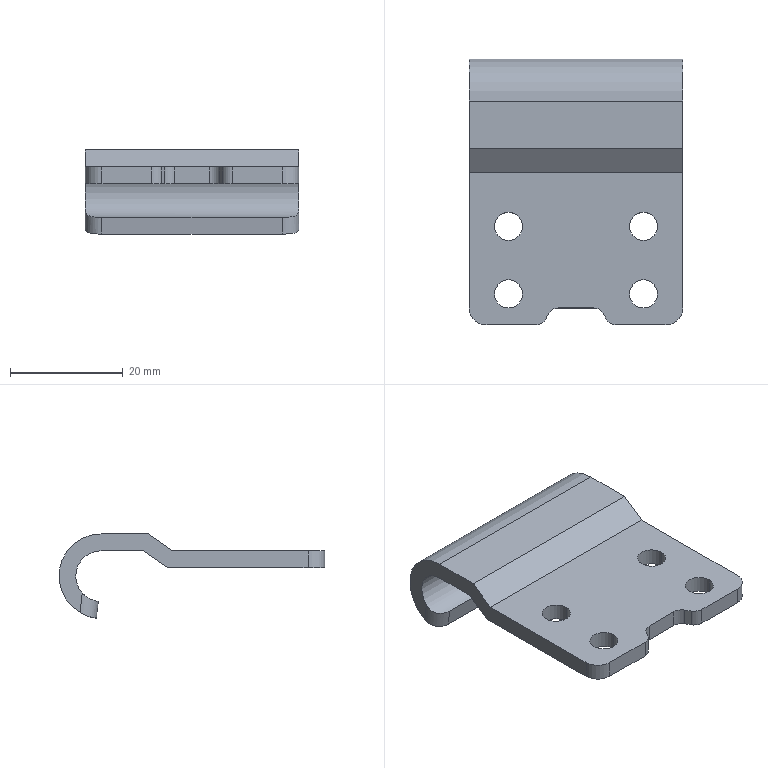Part | SolidWorks | features BaseBody 1 | 1 solid | 32 faces | box 38 x 47.284 x 14.954 mm | volume 6365 mm3 | cylinder 18 | plane 14 | commonest cylinder face diameters 5 x8 4 x4 6 x4 9 x1 15 x1
STEP:
#1=CARTESIAN_POINT('',(-19.,13.284,-5.));
#2=VERTEX_POINT('',#1);
#3=CARTESIAN_POINT('',(19.,13.284,-5.));
#4=VERTEX_POINT('',#3);
#5=CARTESIAN_POINT('',(-19.,13.284,-5.));
#6=DIRECTION('',(1.,0.,0.));
#7=VECTOR('',#6,1000.);
#8=LINE('',#5,#7);
#9=EDGE_CURVE('',#2,#4,#8,.T.);
#10=ORIENTED_EDGE('',*,*,#9,.T.);
#11=CARTESIAN_POINT('',(19.,5.784,-5.));
#12=VERTEX_POINT('',#11);
#13=CARTESIAN_POINT('',(19.,5.784,-5.));
#14=DIRECTION('',(0.,1.,0.));
#15=VECTOR('',#14,1000.);
#16=LINE('',#13,#15);
#17=EDGE_CURVE('',#12,#4,#16,.T.);
#18=ORIENTED_EDGE('',*,*,#17,.F.);
#19=CARTESIAN_POINT('',(-19.,5.784,-5.));
#20=VERTEX_POINT('',#19);
#21=CARTESIAN_POINT('',(19.,5.784,-5.));
#22=DIRECTION('',(-1.,0.,0.));
#23=VECTOR('',#22,1000.);
#24=LINE('',#21,#23);
#25=EDGE_CURVE('',#12,#20,#24,.T.);
#26=ORIENTED_EDGE('',*,*,#25,.T.);
#27=CARTESIAN_POINT('',(-19.,5.784,-5.));
#28=DIRECTION('',(0.,1.,0.));
#29=VECTOR('',#28,1000.);
#30=LINE('',#27,#29);
#31=EDGE_CURVE('',#20,#2,#30,.T.);
#32=ORIENTED_EDGE('',*,*,#31,.T.);
#33=EDGE_LOOP('',(#10,#18,#26,#32));
#34=FACE_OUTER_BOUND('',#33,.T.);
#35=CARTESIAN_POINT('',(19.,17.784,-5.));
#36=DIRECTION('',(0.,0.,-1.));
#37=DIRECTION('',(0.,-1.,0.));
#38=AXIS2_PLACEMENT_3D('',#35,#36,#37);
#39=PLANE('',#38);
#40=ADVANCED_FACE('',(#34),#39,.T.);
#41=CARTESIAN_POINT('',(-19.,-23.5,-8.));
#42=VERTEX_POINT('',#41);
#43=CARTESIAN_POINT('',(-19.,-23.5,-5.));
#44=VERTEX_POINT('',#43);
#45=CARTESIAN_POINT('',(-19.,-23.5,-8.));
#46=DIRECTION('',(0.,0.,1.));
#47=VECTOR('',#46,1000.);
#48=LINE('',#45,#47);
#49=EDGE_CURVE('',#42,#44,#48,.T.);
#50=ORIENTED_EDGE('',*,*,#49,.T.);
#51=CARTESIAN_POINT('',(-19.,0.5541,-5.));
#52=VERTEX_POINT('',#51);
#53=CARTESIAN_POINT('',(-19.,0.5541,-5.));
#54=DIRECTION('',(0.,-1.,0.));
#55=VECTOR('',#54,1000.);
#56=LINE('',#53,#55);
#57=EDGE_CURVE('',#52,#44,#56,.T.);
#58=ORIENTED_EDGE('',*,*,#57,.F.);
#59=CARTESIAN_POINT('',(-19.,4.839,-2.));
#60=VERTEX_POINT('',#59);
#61=CARTESIAN_POINT('',(-19.,4.839,-2.));
#62=DIRECTION('',(0.,-0.8192,-0.5736));
#63=VECTOR('',#62,1000.);
#64=LINE('',#61,#63);
#65=EDGE_CURVE('',#60,#52,#64,.T.);
#66=ORIENTED_EDGE('',*,*,#65,.F.);
#67=CARTESIAN_POINT('',(-19.,13.284,-2.));
#68=VERTEX_POINT('',#67);
#69=CARTESIAN_POINT('',(-19.,13.284,-2.));
#70=DIRECTION('',(0.,-1.,0.));
#71=VECTOR('',#70,1000.);
#72=LINE('',#69,#71);
#73=EDGE_CURVE('',#68,#60,#72,.T.);
#74=ORIENTED_EDGE('',*,*,#73,.F.);
#75=CARTESIAN_POINT('',(-19.,17.03,-15.998));
#76=VERTEX_POINT('',#75);
#77=CARTESIAN_POINT('',(-19.,13.284,-9.5));
#78=DIRECTION('',(1.,0.,0.));
#79=DIRECTION('',(0.,0.4994,-0.8664));
#80=AXIS2_PLACEMENT_3D('',#77,#78,#79);
#81=CIRCLE('',#80,7.5);
#82=EDGE_CURVE('',#76,#68,#81,.T.);
#83=ORIENTED_EDGE('',*,*,#82,.F.);
#84=CARTESIAN_POINT('',(-19.,16.639,-12.5));
#85=VERTEX_POINT('',#84);
#86=CARTESIAN_POINT('',(-19.,16.639,-12.5));
#87=DIRECTION('',(0.,0.1111,-0.9938));
#88=VECTOR('',#87,1000.);
#89=LINE('',#86,#88);
#90=EDGE_CURVE('',#85,#76,#89,.T.);
#91=ORIENTED_EDGE('',*,*,#90,.F.);
#92=CARTESIAN_POINT('',(-19.,13.284,-9.5));
#93=DIRECTION('',(-1.,0.,0.));
#94=DIRECTION('',(0.,0.,1.));
#95=AXIS2_PLACEMENT_3D('',#92,#93,#94);
#96=CIRCLE('',#95,4.5);
#97=EDGE_CURVE('',#2,#85,#96,.T.);
#98=ORIENTED_EDGE('',*,*,#97,.F.);
#99=ORIENTED_EDGE('',*,*,#31,.F.);
#100=CARTESIAN_POINT('',(-19.,1.5,-8.));
#101=VERTEX_POINT('',#100);
#102=CARTESIAN_POINT('',(-19.,1.5,-8.));
#103=DIRECTION('',(0.,0.8192,0.5736));
#104=VECTOR('',#103,1000.);
#105=LINE('',#102,#104);
#106=EDGE_CURVE('',#101,#20,#105,.T.);
#107=ORIENTED_EDGE('',*,*,#106,.F.);
#108=CARTESIAN_POINT('',(-19.,1.5,-8.));
#109=DIRECTION('',(0.,-1.,0.));
#110=VECTOR('',#109,1000.);
#111=LINE('',#108,#110);
#112=EDGE_CURVE('',#101,#42,#111,.T.);
#113=ORIENTED_EDGE('',*,*,#112,.T.);
#114=EDGE_LOOP('',(#50,#58,#66,#74,#83,#91,#98,#99,#107,#113));
#115=FACE_OUTER_BOUND('',#114,.T.);
#116=CARTESIAN_POINT('',(-19.,25.784,200.273));
#117=DIRECTION('',(-1.,0.,0.));
#118=DIRECTION('',(0.,0.,1.));
#119=AXIS2_PLACEMENT_3D('',#116,#117,#118);
#120=PLANE('',#119);
#121=ADVANCED_FACE('',(#115),#120,.T.);
#122=CARTESIAN_POINT('',(-9.5,-9.,-8.));
#123=VERTEX_POINT('',#122);
#124=CARTESIAN_POINT('',(-14.5,-9.,-8.));
#125=VERTEX_POINT('',#124);
#126=CARTESIAN_POINT('',(-12.,-9.,-8.));
#127=DIRECTION('',(0.,0.,-1.));
#128=DIRECTION('',(1.,0.,0.));
#129=AXIS2_PLACEMENT_3D('',#126,#127,#128);
#130=CIRCLE('',#129,2.5);
#131=EDGE_CURVE('',#123,#125,#130,.T.);
#132=ORIENTED_EDGE('',*,*,#131,.F.);
#133=CARTESIAN_POINT('',(-12.,-9.,-8.));
#134=DIRECTION('',(0.,0.,-1.));
#135=DIRECTION('',(-1.,0.,0.));
#136=AXIS2_PLACEMENT_3D('',#133,#134,#135);
#137=CIRCLE('',#136,2.5);
#138=EDGE_CURVE('',#125,#123,#137,.T.);
#139=ORIENTED_EDGE('',*,*,#138,.F.);
#140=EDGE_LOOP('',(#132,#139));
#141=FACE_BOUND('',#140,.T.);
#142=CARTESIAN_POINT('',(-9.5,-21.,-8.));
#143=VERTEX_POINT('',#142);
#144=CARTESIAN_POINT('',(-14.5,-21.,-8.));
#145=VERTEX_POINT('',#144);
#146=CARTESIAN_POINT('',(-12.,-21.,-8.));
#147=DIRECTION('',(0.,0.,-1.));
#148=DIRECTION('',(1.,0.,0.));
#149=AXIS2_PLACEMENT_3D('',#146,#147,#148);
#150=CIRCLE('',#149,2.5);
#151=EDGE_CURVE('',#143,#145,#150,.T.);
#152=ORIENTED_EDGE('',*,*,#151,.F.);
#153=CARTESIAN_POINT('',(-12.,-21.,-8.));
#154=DIRECTION('',(0.,0.,-1.));
#155=DIRECTION('',(-1.,0.,0.));
#156=AXIS2_PLACEMENT_3D('',#153,#154,#155);
#157=CIRCLE('',#156,2.5);
#158=EDGE_CURVE('',#145,#143,#157,.T.);
#159=ORIENTED_EDGE('',*,*,#158,.F.);
#160=EDGE_LOOP('',(#152,#159));
#161=FACE_BOUND('',#160,.T.);
#162=CARTESIAN_POINT('',(14.5,-9.,-8.));
#163=VERTEX_POINT('',#162);
#164=CARTESIAN_POINT('',(9.5,-9.,-8.));
#165=VERTEX_POINT('',#164);
#166=CARTESIAN_POINT('',(12.,-9.,-8.));
#167=DIRECTION('',(0.,0.,-1.));
#168=DIRECTION('',(1.,0.,0.));
#169=AXIS2_PLACEMENT_3D('',#166,#167,#168);
#170=CIRCLE('',#169,2.5);
#171=EDGE_CURVE('',#163,#165,#170,.T.);
#172=ORIENTED_EDGE('',*,*,#171,.F.);
#173=CARTESIAN_POINT('',(12.,-9.,-8.));
#174=DIRECTION('',(0.,0.,-1.));
#175=DIRECTION('',(-1.,0.,0.));
#176=AXIS2_PLACEMENT_3D('',#173,#174,#175);
#177=CIRCLE('',#176,2.5);
#178=EDGE_CURVE('',#165,#163,#177,.T.);
#179=ORIENTED_EDGE('',*,*,#178,.F.);
#180=EDGE_LOOP('',(#172,#179));
#181=FACE_BOUND('',#180,.T.);
#182=CARTESIAN_POINT('',(14.5,-21.,-8.));
#183=VERTEX_POINT('',#182);
#184=CARTESIAN_POINT('',(9.5,-21.,-8.));
#185=VERTEX_POINT('',#184);
#186=CARTESIAN_POINT('',(12.,-21.,-8.));
#187=DIRECTION('',(0.,0.,-1.));
#188=DIRECTION('',(1.,0.,0.));
#189=AXIS2_PLACEMENT_3D('',#186,#187,#188);
#190=CIRCLE('',#189,2.5);
#191=EDGE_CURVE('',#183,#185,#190,.T.);
#192=ORIENTED_EDGE('',*,*,#191,.F.);
#193=CARTESIAN_POINT('',(12.,-21.,-8.));
#194=DIRECTION('',(0.,0.,-1.));
#195=DIRECTION('',(-1.,0.,0.));
#196=AXIS2_PLACEMENT_3D('',#193,#194,#195);
#197=CIRCLE('',#196,2.5);
#198=EDGE_CURVE('',#185,#183,#197,.T.);
#199=ORIENTED_EDGE('',*,*,#198,.F.);
#200=EDGE_LOOP('',(#192,#199));
#201=FACE_BOUND('',#200,.T.);
#202=CARTESIAN_POINT('',(-16.,-26.5,-8.));
#203=VERTEX_POINT('',#202);
#204=CARTESIAN_POINT('',(-16.,-23.5,-8.));
#205=DIRECTION('',(0.,0.,1.));
#206=DIRECTION('',(-1.,0.,0.));
#207=AXIS2_PLACEMENT_3D('',#204,#205,#206);
#208=CIRCLE('',#207,3.);
#209=EDGE_CURVE('',#42,#203,#208,.T.);
#210=ORIENTED_EDGE('',*,*,#209,.F.);
#211=ORIENTED_EDGE('',*,*,#112,.F.);
#212=CARTESIAN_POINT('',(19.,1.5,-8.));
#213=VERTEX_POINT('',#212);
#214=CARTESIAN_POINT('',(19.,1.5,-8.));
#215=DIRECTION('',(-1.,0.,0.));
#216=VECTOR('',#215,1000.);
#217=LINE('',#214,#216);
#218=EDGE_CURVE('',#213,#101,#217,.T.);
#219=ORIENTED_EDGE('',*,*,#218,.F.);
#220=CARTESIAN_POINT('',(19.,-23.5,-8.));
#221=VERTEX_POINT('',#220);
#222=CARTESIAN_POINT('',(19.,-23.5,-8.));
#223=DIRECTION('',(0.,1.,0.));
#224=VECTOR('',#223,1000.);
#225=LINE('',#222,#224);
#226=EDGE_CURVE('',#221,#213,#225,.T.);
#227=ORIENTED_EDGE('',*,*,#226,.F.);
#228=CARTESIAN_POINT('',(16.,-26.5,-8.));
#229=VERTEX_POINT('',#228);
#230=CARTESIAN_POINT('',(16.,-23.5,-8.));
#231=DIRECTION('',(0.,0.,1.));
#232=DIRECTION('',(0.,-1.,0.));
#233=AXIS2_PLACEMENT_3D('',#230,#231,#232);
#234=CIRCLE('',#233,3.);
#235=EDGE_CURVE('',#229,#221,#234,.T.);
#236=ORIENTED_EDGE('',*,*,#235,.F.);
#237=CARTESIAN_POINT('',(7.155,-26.5,-8.));
#238=VERTEX_POINT('',#237);
#239=CARTESIAN_POINT('',(7.155,-26.5,-8.));
#240=DIRECTION('',(1.,0.,0.));
#241=VECTOR('',#240,1000.);
#242=LINE('',#239,#241);
#243=EDGE_CURVE('',#238,#229,#242,.T.);
#244=ORIENTED_EDGE('',*,*,#243,.F.);
#245=CARTESIAN_POINT('',(5.423,-25.5,-8.));
#246=VERTEX_POINT('',#245);
#247=CARTESIAN_POINT('',(7.155,-24.5,-8.));
#248=DIRECTION('',(0.,0.,1.));
#249=DIRECTION('',(-0.866,-0.5,0.));
#250=AXIS2_PLACEMENT_3D('',#247,#248,#249);
#251=CIRCLE('',#250,2.);
#252=EDGE_CURVE('',#246,#238,#251,.T.);
#253=ORIENTED_EDGE('',*,*,#252,.F.);
#254=CARTESIAN_POINT('',(4.845,-24.5,-8.));
#255=VERTEX_POINT('',#254);
#256=CARTESIAN_POINT('',(4.845,-24.5,-8.));
#257=DIRECTION('',(0.5,-0.866,0.));
#258=VECTOR('',#257,1000.);
#259=LINE('',#256,#258);
#260=EDGE_CURVE('',#255,#246,#259,.T.);
#261=ORIENTED_EDGE('',*,*,#260,.F.);
#262=CARTESIAN_POINT('',(3.113,-23.5,-8.));
#263=VERTEX_POINT('',#262);
#264=CARTESIAN_POINT('',(3.113,-25.5,-8.));
#265=DIRECTION('',(0.,0.,-1.));
#266=DIRECTION('',(0.,1.,0.));
#267=AXIS2_PLACEMENT_3D('',#264,#265,#266);
#268=CIRCLE('',#267,2.);
#269=EDGE_CURVE('',#263,#255,#268,.T.);
#270=ORIENTED_EDGE('',*,*,#269,.F.);
#271=CARTESIAN_POINT('',(-3.113,-23.5,-8.));
#272=VERTEX_POINT('',#271);
#273=CARTESIAN_POINT('',(-3.113,-23.5,-8.));
#274=DIRECTION('',(1.,0.,0.));
#275=VECTOR('',#274,1000.);
#276=LINE('',#273,#275);
#277=EDGE_CURVE('',#272,#263,#276,.T.);
#278=ORIENTED_EDGE('',*,*,#277,.F.);
#279=CARTESIAN_POINT('',(-4.845,-24.5,-8.));
#280=VERTEX_POINT('',#279);
#281=CARTESIAN_POINT('',(-3.113,-25.5,-8.));
#282=DIRECTION('',(0.,0.,-1.));
#283=DIRECTION('',(-0.866,0.5,0.));
#284=AXIS2_PLACEMENT_3D('',#281,#282,#283);
#285=CIRCLE('',#284,2.);
#286=EDGE_CURVE('',#280,#272,#285,.T.);
#287=ORIENTED_EDGE('',*,*,#286,.F.);
#288=CARTESIAN_POINT('',(-5.423,-25.5,-8.));
#289=VERTEX_POINT('',#288);
#290=CARTESIAN_POINT('',(-5.423,-25.5,-8.));
#291=DIRECTION('',(0.5,0.866,0.));
#292=VECTOR('',#291,1000.);
#293=LINE('',#290,#292);
#294=EDGE_CURVE('',#289,#280,#293,.T.);
#295=ORIENTED_EDGE('',*,*,#294,.F.);
#296=CARTESIAN_POINT('',(-7.155,-26.5,-8.));
#297=VERTEX_POINT('',#296);
#298=CARTESIAN_POINT('',(-7.155,-24.5,-8.));
#299=DIRECTION('',(0.,0.,1.));
#300=DIRECTION('',(0.,-1.,0.));
#301=AXIS2_PLACEMENT_3D('',#298,#299,#300);
#302=CIRCLE('',#301,2.);
#303=EDGE_CURVE('',#297,#289,#302,.T.);
#304=ORIENTED_EDGE('',*,*,#303,.F.);
#305=CARTESIAN_POINT('',(-16.,-26.5,-8.));
#306=DIRECTION('',(1.,0.,0.));
#307=VECTOR('',#306,1000.);
#308=LINE('',#305,#307);
#309=EDGE_CURVE('',#203,#297,#308,.T.);
#310=ORIENTED_EDGE('',*,*,#309,.F.);
#311=EDGE_LOOP('',(#210,#211,#219,#227,#236,#244,#253,#261,#270,#278,#287,#295,#304,#310));
#312=FACE_OUTER_BOUND('',#311,.T.);
#313=CARTESIAN_POINT('',(19.,1.5,-8.));
#314=DIRECTION('',(0.,0.,-1.));
#315=DIRECTION('',(0.,-1.,0.));
#316=AXIS2_PLACEMENT_3D('',#313,#314,#315);
#317=PLANE('',#316);
#318=ADVANCED_FACE('',(#141,#161,#181,#201,#312),#317,.T.);
#319=CARTESIAN_POINT('',(-16.,-26.5,-5.));
#320=VERTEX_POINT('',#319);
#321=CARTESIAN_POINT('',(-16.,-26.5,-5.));
#322=DIRECTION('',(0.,0.,-1.));
#323=VECTOR('',#322,1000.);
#324=LINE('',#321,#323);
#325=EDGE_CURVE('',#320,#203,#324,.T.);
#326=ORIENTED_EDGE('',*,*,#325,.T.);
#327=ORIENTED_EDGE('',*,*,#309,.T.);
#328=CARTESIAN_POINT('',(-7.155,-26.5,-5.));
#329=VERTEX_POINT('',#328);
#330=CARTESIAN_POINT('',(-7.155,-26.5,-8.));
#331=DIRECTION('',(0.,0.,1.));
#332=VECTOR('',#331,1000.);
#333=LINE('',#330,#332);
#334=EDGE_CURVE('',#297,#329,#333,.T.);
#335=ORIENTED_EDGE('',*,*,#334,.T.);
#336=CARTESIAN_POINT('',(-16.,-26.5,-5.));
#337=DIRECTION('',(1.,0.,0.));
#338=VECTOR('',#337,1000.);
#339=LINE('',#336,#338);
#340=EDGE_CURVE('',#320,#329,#339,.T.);
#341=ORIENTED_EDGE('',*,*,#340,.F.);
#342=EDGE_LOOP('',(#326,#327,#335,#341));
#343=FACE_OUTER_BOUND('',#342,.T.);
#344=CARTESIAN_POINT('',(19.,-26.5,-8.));
#345=DIRECTION('',(0.,-1.,0.));
#346=DIRECTION('',(0.,0.,-1.));
#347=AXIS2_PLACEMENT_3D('',#344,#345,#346);
#348=PLANE('',#347);
#349=ADVANCED_FACE('',(#343),#348,.T.);
#350=CARTESIAN_POINT('',(-9.5,-9.,-5.));
#351=VERTEX_POINT('',#350);
#352=CARTESIAN_POINT('',(-14.5,-9.,-5.));
#353=VERTEX_POINT('',#352);
#354=CARTESIAN_POINT('',(-12.,-9.,-5.));
#355=DIRECTION('',(0.,0.,1.));
#356=DIRECTION('',(1.,0.,0.));
#357=AXIS2_PLACEMENT_3D('',#354,#355,#356);
#358=CIRCLE('',#357,2.5);
#359=EDGE_CURVE('',#351,#353,#358,.T.);
#360=ORIENTED_EDGE('',*,*,#359,.F.);
#361=CARTESIAN_POINT('',(-12.,-9.,-5.));
#362=DIRECTION('',(0.,0.,1.));
#363=DIRECTION('',(-1.,0.,0.));
#364=AXIS2_PLACEMENT_3D('',#361,#362,#363);
#365=CIRCLE('',#364,2.5);
#366=EDGE_CURVE('',#353,#351,#365,.T.);
#367=ORIENTED_EDGE('',*,*,#366,.F.);
#368=EDGE_LOOP('',(#360,#367));
#369=FACE_BOUND('',#368,.T.);
#370=CARTESIAN_POINT('',(-9.5,-21.,-5.));
#371=VERTEX_POINT('',#370);
#372=CARTESIAN_POINT('',(-14.5,-21.,-5.));
#373=VERTEX_POINT('',#372);
#374=CARTESIAN_POINT('',(-12.,-21.,-5.));
#375=DIRECTION('',(0.,0.,1.));
#376=DIRECTION('',(1.,0.,0.));
#377=AXIS2_PLACEMENT_3D('',#374,#375,#376);
#378=CIRCLE('',#377,2.5);
#379=EDGE_CURVE('',#371,#373,#378,.T.);
#380=ORIENTED_EDGE('',*,*,#379,.F.);
#381=CARTESIAN_POINT('',(-12.,-21.,-5.));
#382=DIRECTION('',(0.,0.,1.));
#383=DIRECTION('',(-1.,0.,0.));
#384=AXIS2_PLACEMENT_3D('',#381,#382,#383);
#385=CIRCLE('',#384,2.5);
#386=EDGE_CURVE('',#373,#371,#385,.T.);
#387=ORIENTED_EDGE('',*,*,#386,.F.);
#388=EDGE_LOOP('',(#380,#387));
#389=FACE_BOUND('',#388,.T.);
#390=CARTESIAN_POINT('',(14.5,-9.,-5.));
#391=VERTEX_POINT('',#390);
#392=CARTESIAN_POINT('',(9.5,-9.,-5.));
#393=VERTEX_POINT('',#392);
#394=CARTESIAN_POINT('',(12.,-9.,-5.));
#395=DIRECTION('',(0.,0.,1.));
#396=DIRECTION('',(1.,0.,0.));
#397=AXIS2_PLACEMENT_3D('',#394,#395,#396);
#398=CIRCLE('',#397,2.5);
#399=EDGE_CURVE('',#391,#393,#398,.T.);
#400=ORIENTED_EDGE('',*,*,#399,.F.);
#401=CARTESIAN_POINT('',(12.,-9.,-5.));
#402=DIRECTION('',(0.,0.,1.));
#403=DIRECTION('',(-1.,0.,0.));
#404=AXIS2_PLACEMENT_3D('',#401,#402,#403);
#405=CIRCLE('',#404,2.5);
#406=EDGE_CURVE('',#393,#391,#405,.T.);
#407=ORIENTED_EDGE('',*,*,#406,.F.);
#408=EDGE_LOOP('',(#400,#407));
#409=FACE_BOUND('',#408,.T.);
#410=CARTESIAN_POINT('',(14.5,-21.,-5.));
#411=VERTEX_POINT('',#410);
#412=CARTESIAN_POINT('',(9.5,-21.,-5.));
#413=VERTEX_POINT('',#412);
#414=CARTESIAN_POINT('',(12.,-21.,-5.));
#415=DIRECTION('',(0.,0.,1.));
#416=DIRECTION('',(1.,0.,0.));
#417=AXIS2_PLACEMENT_3D('',#414,#415,#416);
#418=CIRCLE('',#417,2.5);
#419=EDGE_CURVE('',#411,#413,#418,.T.);
#420=ORIENTED_EDGE('',*,*,#419,.F.);
#421=CARTESIAN_POINT('',(12.,-21.,-5.));
#422=DIRECTION('',(0.,0.,1.));
#423=DIRECTION('',(-1.,0.,0.));
#424=AXIS2_PLACEMENT_3D('',#421,#422,#423);
#425=CIRCLE('',#424,2.5);
#426=EDGE_CURVE('',#413,#411,#425,.T.);
#427=ORIENTED_EDGE('',*,*,#426,.F.);
#428=EDGE_LOOP('',(#420,#427));
#429=FACE_BOUND('',#428,.T.);
#430=CARTESIAN_POINT('',(-16.,-23.5,-5.));
#431=DIRECTION('',(0.,0.,-1.));
#432=DIRECTION('',(0.,-1.,0.));
#433=AXIS2_PLACEMENT_3D('',#430,#431,#432);
#434=CIRCLE('',#433,3.);
#435=EDGE_CURVE('',#320,#44,#434,.T.);
#436=ORIENTED_EDGE('',*,*,#435,.F.);
#437=ORIENTED_EDGE('',*,*,#340,.T.);
#438=CARTESIAN_POINT('',(-5.423,-25.5,-5.));
#439=VERTEX_POINT('',#438);
#440=CARTESIAN_POINT('',(-7.155,-24.5,-5.));
#441=DIRECTION('',(0.,0.,-1.));
#442=DIRECTION('',(0.866,-0.5,0.));
#443=AXIS2_PLACEMENT_3D('',#440,#441,#442);
#444=CIRCLE('',#443,2.);
#445=EDGE_CURVE('',#439,#329,#444,.T.);
#446=ORIENTED_EDGE('',*,*,#445,.F.);
#447=CARTESIAN_POINT('',(-4.845,-24.5,-5.));
#448=VERTEX_POINT('',#447);
#449=CARTESIAN_POINT('',(-4.845,-24.5,-5.));
#450=DIRECTION('',(-0.5,-0.866,0.));
#451=VECTOR('',#450,1000.);
#452=LINE('',#449,#451);
#453=EDGE_CURVE('',#448,#439,#452,.T.);
#454=ORIENTED_EDGE('',*,*,#453,.F.);
#455=CARTESIAN_POINT('',(-3.113,-23.5,-5.));
#456=VERTEX_POINT('',#455);
#457=CARTESIAN_POINT('',(-3.113,-25.5,-5.));
#458=DIRECTION('',(0.,0.,1.));
#459=DIRECTION('',(0.,1.,0.));
#460=AXIS2_PLACEMENT_3D('',#457,#458,#459);
#461=CIRCLE('',#460,2.);
#462=EDGE_CURVE('',#456,#448,#461,.T.);
#463=ORIENTED_EDGE('',*,*,#462,.F.);
#464=CARTESIAN_POINT('',(3.113,-23.5,-5.));
#465=VERTEX_POINT('',#464);
#466=CARTESIAN_POINT('',(3.113,-23.5,-5.));
#467=DIRECTION('',(-1.,0.,0.));
#468=VECTOR('',#467,1000.);
#469=LINE('',#466,#468);
#470=EDGE_CURVE('',#465,#456,#469,.T.);
#471=ORIENTED_EDGE('',*,*,#470,.F.);
#472=CARTESIAN_POINT('',(4.845,-24.5,-5.));
#473=VERTEX_POINT('',#472);
#474=CARTESIAN_POINT('',(3.113,-25.5,-5.));
#475=DIRECTION('',(0.,0.,1.));
#476=DIRECTION('',(0.866,0.5,0.));
#477=AXIS2_PLACEMENT_3D('',#474,#475,#476);
#478=CIRCLE('',#477,2.);
#479=EDGE_CURVE('',#473,#465,#478,.T.);
#480=ORIENTED_EDGE('',*,*,#479,.F.);
#481=CARTESIAN_POINT('',(5.423,-25.5,-5.));
#482=VERTEX_POINT('',#481);
#483=CARTESIAN_POINT('',(5.423,-25.5,-5.));
#484=DIRECTION('',(-0.5,0.866,0.));
#485=VECTOR('',#484,1000.);
#486=LINE('',#483,#485);
#487=EDGE_CURVE('',#482,#473,#486,.T.);
#488=ORIENTED_EDGE('',*,*,#487,.F.);
#489=CARTESIAN_POINT('',(7.155,-26.5,-5.));
#490=VERTEX_POINT('',#489);
#491=CARTESIAN_POINT('',(7.155,-24.5,-5.));
#492=DIRECTION('',(0.,0.,-1.));
#493=DIRECTION('',(0.,-1.,0.));
#494=AXIS2_PLACEMENT_3D('',#491,#492,#493);
#495=CIRCLE('',#494,2.);
#496=EDGE_CURVE('',#490,#482,#495,.T.);
#497=ORIENTED_EDGE('',*,*,#496,.F.);
#498=CARTESIAN_POINT('',(16.,-26.5,-5.));
#499=VERTEX_POINT('',#498);
#500=CARTESIAN_POINT('',(7.155,-26.5,-5.));
#501=DIRECTION('',(1.,0.,0.));
#502=VECTOR('',#501,1000.);
#503=LINE('',#500,#502);
#504=EDGE_CURVE('',#490,#499,#503,.T.);
#505=ORIENTED_EDGE('',*,*,#504,.T.);
#506=CARTESIAN_POINT('',(19.,-23.5,-5.));
#507=VERTEX_POINT('',#506);
#508=CARTESIAN_POINT('',(16.,-23.5,-5.));
#509=DIRECTION('',(0.,0.,-1.));
#510=DIRECTION('',(1.,0.,0.));
#511=AXIS2_PLACEMENT_3D('',#508,#509,#510);
#512=CIRCLE('',#511,3.);
#513=EDGE_CURVE('',#507,#499,#512,.T.);
#514=ORIENTED_EDGE('',*,*,#513,.F.);
#515=CARTESIAN_POINT('',(19.,0.5541,-5.));
#516=VERTEX_POINT('',#515);
#517=CARTESIAN_POINT('',(19.,0.5541,-5.));
#518=DIRECTION('',(0.,-1.,0.));
#519=VECTOR('',#518,1000.);
#520=LINE('',#517,#519);
#521=EDGE_CURVE('',#516,#507,#520,.T.);
#522=ORIENTED_EDGE('',*,*,#521,.F.);
#523=CARTESIAN_POINT('',(-19.,0.5541,-5.));
#524=DIRECTION('',(1.,0.,0.));
#525=VECTOR('',#524,1000.);
#526=LINE('',#523,#525);
#527=EDGE_CURVE('',#52,#516,#526,.T.);
#528=ORIENTED_EDGE('',*,*,#527,.F.);
#529=ORIENTED_EDGE('',*,*,#57,.T.);
#530=EDGE_LOOP('',(#436,#437,#446,#454,#463,#471,#480,#488,#497,#505,#514,#522,#528,#529));
#531=FACE_OUTER_BOUND('',#530,.T.);
#532=CARTESIAN_POINT('',(19.,-26.5,-5.));
#533=DIRECTION('',(0.,0.,1.));
#534=DIRECTION('',(1.,0.,0.));
#535=AXIS2_PLACEMENT_3D('',#532,#533,#534);
#536=PLANE('',#535);
#537=ADVANCED_FACE('',(#369,#389,#409,#429,#531),#536,.T.);
#538=CARTESIAN_POINT('',(19.,4.839,-2.));
#539=VERTEX_POINT('',#538);
#540=CARTESIAN_POINT('',(19.,0.5541,-5.));
#541=DIRECTION('',(0.,0.8192,0.5736));
#542=VECTOR('',#541,1000.);
#543=LINE('',#540,#542);
#544=EDGE_CURVE('',#516,#539,#543,.T.);
#545=ORIENTED_EDGE('',*,*,#544,.T.);
#546=CARTESIAN_POINT('',(19.,4.839,-2.));
#547=DIRECTION('',(-1.,0.,0.));
#548=VECTOR('',#547,1000.);
#549=LINE('',#546,#548);
#550=EDGE_CURVE('',#539,#60,#549,.T.);
#551=ORIENTED_EDGE('',*,*,#550,.T.);
#552=ORIENTED_EDGE('',*,*,#65,.T.);
#553=ORIENTED_EDGE('',*,*,#527,.T.);
#554=EDGE_LOOP('',(#545,#551,#552,#553));
#555=FACE_OUTER_BOUND('',#554,.T.);
#556=CARTESIAN_POINT('',(19.,0.5541,-5.));
#557=DIRECTION('',(0.,-0.5736,0.8192));
#558=DIRECTION('',(-1.,0.,0.));
#559=AXIS2_PLACEMENT_3D('',#556,#557,#558);
#560=PLANE('',#559);
#561=ADVANCED_FACE('',(#555),#560,.T.);
#562=CARTESIAN_POINT('',(19.,13.284,-2.));
#563=VERTEX_POINT('',#562);
#564=CARTESIAN_POINT('',(19.,13.284,-2.));
#565=DIRECTION('',(-1.,0.,0.));
#566=VECTOR('',#565,1000.);
#567=LINE('',#564,#566);
#568=EDGE_CURVE('',#563,#68,#567,.T.);
#569=ORIENTED_EDGE('',*,*,#568,.T.);
#570=ORIENTED_EDGE('',*,*,#73,.T.);
#571=ORIENTED_EDGE('',*,*,#550,.F.);
#572=CARTESIAN_POINT('',(19.,13.284,-2.));
#573=DIRECTION('',(0.,-1.,0.));
#574=VECTOR('',#573,1000.);
#575=LINE('',#572,#574);
#576=EDGE_CURVE('',#563,#539,#575,.T.);
#577=ORIENTED_EDGE('',*,*,#576,.F.);
#578=EDGE_LOOP('',(#569,#570,#571,#577));
#579=FACE_OUTER_BOUND('',#578,.T.);
#580=CARTESIAN_POINT('',(19.,4.839,-2.));
#581=DIRECTION('',(0.,0.,1.));
#582=DIRECTION('',(1.,0.,0.));
#583=AXIS2_PLACEMENT_3D('',#580,#581,#582);
#584=PLANE('',#583);
#585=ADVANCED_FACE('',(#579),#584,.T.);
#586=ORIENTED_EDGE('',*,*,#17,.T.);
#587=CARTESIAN_POINT('',(19.,16.639,-12.5));
#588=VERTEX_POINT('',#587);
#589=CARTESIAN_POINT('',(19.,13.284,-9.5));
#590=DIRECTION('',(1.,0.,0.));
#591=DIRECTION('',(0.,0.7454,-0.6667));
#592=AXIS2_PLACEMENT_3D('',#589,#590,#591);
#593=CIRCLE('',#592,4.5);
#594=EDGE_CURVE('',#588,#4,#593,.T.);
#595=ORIENTED_EDGE('',*,*,#594,.F.);
#596=CARTESIAN_POINT('',(19.,17.03,-15.998));
#597=VERTEX_POINT('',#596);
#598=CARTESIAN_POINT('',(19.,17.03,-15.998));
#599=DIRECTION('',(0.,-0.1111,0.9938));
#600=VECTOR('',#599,1000.);
#601=LINE('',#598,#600);
#602=EDGE_CURVE('',#597,#588,#601,.T.);
#603=ORIENTED_EDGE('',*,*,#602,.F.);
#604=CARTESIAN_POINT('',(19.,13.284,-9.5));
#605=DIRECTION('',(-1.,0.,0.));
#606=DIRECTION('',(0.,0.,1.));
#607=AXIS2_PLACEMENT_3D('',#604,#605,#606);
#608=CIRCLE('',#607,7.5);
#609=EDGE_CURVE('',#563,#597,#608,.T.);
#610=ORIENTED_EDGE('',*,*,#609,.F.);
#611=ORIENTED_EDGE('',*,*,#576,.T.);
#612=ORIENTED_EDGE('',*,*,#544,.F.);
#613=ORIENTED_EDGE('',*,*,#521,.T.);
#614=CARTESIAN_POINT('',(19.,-23.5,-5.));
#615=DIRECTION('',(0.,0.,-1.));
#616=VECTOR('',#615,1000.);
#617=LINE('',#614,#616);
#618=EDGE_CURVE('',#507,#221,#617,.T.);
#619=ORIENTED_EDGE('',*,*,#618,.T.);
#620=ORIENTED_EDGE('',*,*,#226,.T.);
#621=CARTESIAN_POINT('',(19.,5.784,-5.));
#622=DIRECTION('',(0.,-0.8192,-0.5736));
#623=VECTOR('',#622,1000.);
#624=LINE('',#621,#623);
#625=EDGE_CURVE('',#12,#213,#624,.T.);
#626=ORIENTED_EDGE('',*,*,#625,.F.);
#627=EDGE_LOOP('',(#586,#595,#603,#610,#611,#612,#613,#619,#620,#626));
#628=FACE_OUTER_BOUND('',#627,.T.);
#629=CARTESIAN_POINT('',(19.,25.784,200.273));
#630=DIRECTION('',(-1.,0.,0.));
#631=DIRECTION('',(0.,0.,1.));
#632=AXIS2_PLACEMENT_3D('',#629,#630,#631);
#633=PLANE('',#632);
#634=ADVANCED_FACE('',(#628),#633,.F.);
#635=ORIENTED_EDGE('',*,*,#625,.T.);
#636=ORIENTED_EDGE('',*,*,#218,.T.);
#637=ORIENTED_EDGE('',*,*,#106,.T.);
#638=ORIENTED_EDGE('',*,*,#25,.F.);
#639=EDGE_LOOP('',(#635,#636,#637,#638));
#640=FACE_OUTER_BOUND('',#639,.T.);
#641=CARTESIAN_POINT('',(19.,5.784,-5.));
#642=DIRECTION('',(0.,0.5736,-0.8192));
#643=DIRECTION('',(-1.,0.,0.));
#644=AXIS2_PLACEMENT_3D('',#641,#642,#643);
#645=PLANE('',#644);
#646=ADVANCED_FACE('',(#640),#645,.T.);
#647=CARTESIAN_POINT('',(16.,-26.5,-8.));
#648=DIRECTION('',(0.,0.,1.));
#649=VECTOR('',#648,1000.);
#650=LINE('',#647,#649);
#651=EDGE_CURVE('',#229,#499,#650,.T.);
#652=ORIENTED_EDGE('',*,*,#651,.F.);
#653=ORIENTED_EDGE('',*,*,#235,.T.);
#654=ORIENTED_EDGE('',*,*,#618,.F.);
#655=ORIENTED_EDGE('',*,*,#513,.T.);
#656=EDGE_LOOP('',(#652,#653,#654,#655));
#657=FACE_OUTER_BOUND('',#656,.T.);
#658=CARTESIAN_POINT('',(16.,-23.5,-4.463));
#659=DIRECTION('',(0.,0.,-1.));
#660=DIRECTION('',(1.,0.,0.));
#661=AXIS2_PLACEMENT_3D('',#658,#659,#660);
#662=CYLINDRICAL_SURFACE('',#661,3.);
#663=ADVANCED_FACE('',(#657),#662,.T.);
#664=ORIENTED_EDGE('',*,*,#651,.T.);
#665=ORIENTED_EDGE('',*,*,#504,.F.);
#666=CARTESIAN_POINT('',(7.155,-26.5,-5.));
#667=DIRECTION('',(0.,0.,-1.));
#668=VECTOR('',#667,1000.);
#669=LINE('',#666,#668);
#670=EDGE_CURVE('',#490,#238,#669,.T.);
#671=ORIENTED_EDGE('',*,*,#670,.T.);
#672=ORIENTED_EDGE('',*,*,#243,.T.);
#673=EDGE_LOOP('',(#664,#665,#671,#672));
#674=FACE_OUTER_BOUND('',#673,.T.);
#675=CARTESIAN_POINT('',(19.,-26.5,-8.));
#676=DIRECTION('',(0.,-1.,0.));
#677=DIRECTION('',(0.,0.,-1.));
#678=AXIS2_PLACEMENT_3D('',#675,#676,#677);
#679=PLANE('',#678);
#680=ADVANCED_FACE('',(#674),#679,.T.);
#681=CARTESIAN_POINT('',(5.423,-25.5,-8.));
#682=DIRECTION('',(0.,0.,1.));
#683=VECTOR('',#682,1000.);
#684=LINE('',#681,#683);
#685=EDGE_CURVE('',#246,#482,#684,.T.);
#686=ORIENTED_EDGE('',*,*,#685,.F.);
#687=ORIENTED_EDGE('',*,*,#252,.T.);
#688=ORIENTED_EDGE('',*,*,#670,.F.);
#689=ORIENTED_EDGE('',*,*,#496,.T.);
#690=EDGE_LOOP('',(#686,#687,#688,#689));
#691=FACE_OUTER_BOUND('',#690,.T.);
#692=CARTESIAN_POINT('',(7.155,-24.5,-4.672));
#693=DIRECTION('',(0.,0.,-1.));
#694=DIRECTION('',(1.,0.,0.));
#695=AXIS2_PLACEMENT_3D('',#692,#693,#694);
#696=CYLINDRICAL_SURFACE('',#695,2.);
#697=ADVANCED_FACE('',(#691),#696,.T.);
#698=ORIENTED_EDGE('',*,*,#260,.T.);
#699=ORIENTED_EDGE('',*,*,#685,.T.);
#700=ORIENTED_EDGE('',*,*,#487,.T.);
#701=CARTESIAN_POINT('',(4.845,-24.5,-5.));
#702=DIRECTION('',(0.,0.,-1.));
#703=VECTOR('',#702,1000.);
#704=LINE('',#701,#703);
#705=EDGE_CURVE('',#473,#255,#704,.T.);
#706=ORIENTED_EDGE('',*,*,#705,.T.);
#707=EDGE_LOOP('',(#698,#699,#700,#706));
#708=FACE_OUTER_BOUND('',#707,.T.);
#709=CARTESIAN_POINT('',(4.268,-23.5,-8.));
#710=DIRECTION('',(0.866,0.5,0.));
#711=DIRECTION('',(0.,0.,-1.));
#712=AXIS2_PLACEMENT_3D('',#709,#710,#711);
#713=PLANE('',#712);
#714=ADVANCED_FACE('',(#708),#713,.F.);
#715=ORIENTED_EDGE('',*,*,#269,.T.);
#716=ORIENTED_EDGE('',*,*,#705,.F.);
#717=ORIENTED_EDGE('',*,*,#479,.T.);
#718=CARTESIAN_POINT('',(3.113,-23.5,-8.));
#719=DIRECTION('',(0.,0.,1.));
#720=VECTOR('',#719,1000.);
#721=LINE('',#718,#720);
#722=EDGE_CURVE('',#263,#465,#721,.T.);
#723=ORIENTED_EDGE('',*,*,#722,.F.);
#724=EDGE_LOOP('',(#715,#716,#717,#723));
#725=FACE_OUTER_BOUND('',#724,.T.);
#726=CARTESIAN_POINT('',(3.113,-25.5,-8.384));
#727=DIRECTION('',(0.,0.,1.));
#728=DIRECTION('',(-1.,0.,0.));
#729=AXIS2_PLACEMENT_3D('',#726,#727,#728);
#730=CYLINDRICAL_SURFACE('',#729,2.);
#731=ADVANCED_FACE('',(#725),#730,.F.);
#732=ORIENTED_EDGE('',*,*,#277,.T.);
#733=ORIENTED_EDGE('',*,*,#722,.T.);
#734=ORIENTED_EDGE('',*,*,#470,.T.);
#735=CARTESIAN_POINT('',(-3.113,-23.5,-5.));
#736=DIRECTION('',(0.,0.,-1.));
#737=VECTOR('',#736,1000.);
#738=LINE('',#735,#737);
#739=EDGE_CURVE('',#456,#272,#738,.T.);
#740=ORIENTED_EDGE('',*,*,#739,.T.);
#741=EDGE_LOOP('',(#732,#733,#734,#740));
#742=FACE_OUTER_BOUND('',#741,.T.);
#743=CARTESIAN_POINT('',(-4.268,-23.5,-8.));
#744=DIRECTION('',(0.,1.,0.));
#745=DIRECTION('',(1.,0.,0.));
#746=AXIS2_PLACEMENT_3D('',#743,#744,#745);
#747=PLANE('',#746);
#748=ADVANCED_FACE('',(#742),#747,.F.);
#749=ORIENTED_EDGE('',*,*,#286,.T.);
#750=ORIENTED_EDGE('',*,*,#739,.F.);
#751=ORIENTED_EDGE('',*,*,#462,.T.);
#752=CARTESIAN_POINT('',(-4.845,-24.5,-8.));
#753=DIRECTION('',(0.,0.,1.));
#754=VECTOR('',#753,1000.);
#755=LINE('',#752,#754);
#756=EDGE_CURVE('',#280,#448,#755,.T.);
#757=ORIENTED_EDGE('',*,*,#756,.F.);
#758=EDGE_LOOP('',(#749,#750,#751,#757));
#759=FACE_OUTER_BOUND('',#758,.T.);
#760=CARTESIAN_POINT('',(-3.113,-25.5,-8.384));
#761=DIRECTION('',(0.,0.,1.));
#762=DIRECTION('',(-1.,0.,0.));
#763=AXIS2_PLACEMENT_3D('',#760,#761,#762);
#764=CYLINDRICAL_SURFACE('',#763,2.);
#765=ADVANCED_FACE('',(#759),#764,.F.);
#766=ORIENTED_EDGE('',*,*,#453,.T.);
#767=CARTESIAN_POINT('',(-5.423,-25.5,-5.));
#768=DIRECTION('',(0.,0.,-1.));
#769=VECTOR('',#768,1000.);
#770=LINE('',#767,#769);
#771=EDGE_CURVE('',#439,#289,#770,.T.);
#772=ORIENTED_EDGE('',*,*,#771,.T.);
#773=ORIENTED_EDGE('',*,*,#294,.T.);
#774=ORIENTED_EDGE('',*,*,#756,.T.);
#775=EDGE_LOOP('',(#766,#772,#773,#774));
#776=FACE_OUTER_BOUND('',#775,.T.);
#777=CARTESIAN_POINT('',(-6.,-26.5,-8.));
#778=DIRECTION('',(-0.866,0.5,0.));
#779=DIRECTION('',(0.,0.,1.));
#780=AXIS2_PLACEMENT_3D('',#777,#778,#779);
#781=PLANE('',#780);
#782=ADVANCED_FACE('',(#776),#781,.F.);
#783=ORIENTED_EDGE('',*,*,#771,.F.);
#784=ORIENTED_EDGE('',*,*,#445,.T.);
#785=ORIENTED_EDGE('',*,*,#334,.F.);
#786=ORIENTED_EDGE('',*,*,#303,.T.);
#787=EDGE_LOOP('',(#783,#784,#785,#786));
#788=FACE_OUTER_BOUND('',#787,.T.);
#789=CARTESIAN_POINT('',(-7.155,-24.5,-8.396));
#790=DIRECTION('',(0.,0.,1.));
#791=DIRECTION('',(-1.,0.,0.));
#792=AXIS2_PLACEMENT_3D('',#789,#790,#791);
#793=CYLINDRICAL_SURFACE('',#792,2.);
#794=ADVANCED_FACE('',(#788),#793,.T.);
#795=CARTESIAN_POINT('',(-16.,14.118,-16.954));
#796=VERTEX_POINT('',#795);
#797=CARTESIAN_POINT('',(-19.,17.03,-15.998));
#798=CARTESIAN_POINT('',(-19.,16.851,-16.101));
#799=CARTESIAN_POINT('',(-18.982,16.67,-16.195));
#800=CARTESIAN_POINT('',(-18.928,16.401,-16.323));
#801=CARTESIAN_POINT('',(-18.905,16.311,-16.363));
#802=CARTESIAN_POINT('',(-18.864,16.178,-16.42));
#803=CARTESIAN_POINT('',(-18.842,16.111,-16.447));
#804=CARTESIAN_POINT('',(-18.817,16.046,-16.473));
#805=CARTESIAN_POINT('',(-18.8,16.002,-16.491));
#806=CARTESIAN_POINT('',(-18.791,15.978,-16.5));
#807=CARTESIAN_POINT('',(-18.716,15.799,-16.568));
#808=CARTESIAN_POINT('',(-18.631,15.637,-16.623));
#809=CARTESIAN_POINT('',(-18.474,15.398,-16.696));
#810=CARTESIAN_POINT('',(-18.417,15.319,-16.719));
#811=CARTESIAN_POINT('',(-18.323,15.203,-16.75));
#812=CARTESIAN_POINT('',(-18.274,15.145,-16.766));
#813=CARTESIAN_POINT('',(-18.213,15.079,-16.782));
#814=CARTESIAN_POINT('',(-18.182,15.046,-16.79));
#815=CARTESIAN_POINT('',(-18.168,15.032,-16.793));
#816=CARTESIAN_POINT('',(-18.159,15.023,-16.796));
#817=CARTESIAN_POINT('',(-18.154,15.018,-16.797));
#818=CARTESIAN_POINT('',(-18.038,14.901,-16.825));
#819=CARTESIAN_POINT('',(-17.904,14.783,-16.849));
#820=CARTESIAN_POINT('',(-17.663,14.614,-16.881));
#821=CARTESIAN_POINT('',(-17.576,14.559,-16.891));
#822=CARTESIAN_POINT('',(-17.436,14.48,-16.904));
#823=CARTESIAN_POINT('',(-17.388,14.454,-16.908));
#824=CARTESIAN_POINT('',(-17.312,14.417,-16.914));
#825=CARTESIAN_POINT('',(-17.274,14.399,-16.917));
#826=CARTESIAN_POINT('',(-17.228,14.379,-16.92));
#827=CARTESIAN_POINT('',(-17.205,14.368,-16.921));
#828=CARTESIAN_POINT('',(-17.195,14.364,-16.922));
#829=CARTESIAN_POINT('',(-17.189,14.361,-16.922));
#830=CARTESIAN_POINT('',(-17.183,14.359,-16.923));
#831=CARTESIAN_POINT('',(-17.089,14.319,-16.928));
#832=CARTESIAN_POINT('',(-16.947,14.263,-16.936));
#833=CARTESIAN_POINT('',(-16.555,14.162,-16.948));
#834=CARTESIAN_POINT('',(-16.304,14.118,-16.954));
#835=CARTESIAN_POINT('',(-16.,14.118,-16.954));
#836=B_SPLINE_CURVE_WITH_KNOTS('',3,(#797,#798,#799,#800,#801,#802,#803,#804,#805,#806,#807,#808,#809,#810,#811,#812,#813,#814,#815,#816,#817,#818,#819,#820,#821,#822,#823,#824,#825,#826,#827,#828,#829,#830,#831,#832,#833,#834,#835),.UNSPECIFIED.,.F.,.F.,(4,2,2,1,2,2,2,2,1,1,1,2,2,2,2,2,1,1,1,2,2,2,4),(0.,0.125,0.1875,0.2188,0.2344,0.25,0.375,0.4375,0.4688,0.4844,0.4922,0.4961,0.5,0.625,0.6875,0.7188,0.7344,0.7422,0.7461,0.748,0.75,0.875,1.),.UNSPECIFIED.);
#837=EDGE_CURVE('',#76,#796,#836,.T.);
#838=ORIENTED_EDGE('',*,*,#837,.F.);
#839=ORIENTED_EDGE('',*,*,#82,.T.);
#840=ORIENTED_EDGE('',*,*,#568,.F.);
#841=ORIENTED_EDGE('',*,*,#609,.T.);
#842=CARTESIAN_POINT('',(16.,14.118,-16.954));
#843=VERTEX_POINT('',#842);
#844=CARTESIAN_POINT('',(19.,17.03,-15.998));
#845=CARTESIAN_POINT('',(19.,16.846,-16.104));
#846=CARTESIAN_POINT('',(18.982,16.664,-16.198));
#847=CARTESIAN_POINT('',(18.927,16.394,-16.326));
#848=CARTESIAN_POINT('',(18.904,16.305,-16.366));
#849=CARTESIAN_POINT('',(18.849,16.127,-16.441));
#850=CARTESIAN_POINT('',(18.818,16.041,-16.476));
#851=CARTESIAN_POINT('',(18.632,15.598,-16.644));
#852=CARTESIAN_POINT('',(18.416,15.278,-16.736));
#853=CARTESIAN_POINT('',(17.852,14.718,-16.867));
#854=CARTESIAN_POINT('',(17.524,14.499,-16.903));
#855=CARTESIAN_POINT('',(16.788,14.195,-16.946));
#856=CARTESIAN_POINT('',(16.403,14.118,-16.954));
#857=CARTESIAN_POINT('',(16.,14.118,-16.954));
#858=B_SPLINE_CURVE_WITH_KNOTS('',3,(#844,#845,#846,#847,#848,#849,#850,#851,#852,#853,#854,#855,#856,#857),.UNSPECIFIED.,.F.,.F.,(4,2,2,2,2,2,4),(0.,0.125,0.1875,0.25,0.5,0.75,1.),.UNSPECIFIED.);
#859=EDGE_CURVE('',#597,#843,#858,.T.);
#860=ORIENTED_EDGE('',*,*,#859,.T.);
#861=CARTESIAN_POINT('',(-16.,14.118,-16.954));
#862=DIRECTION('',(1.,0.,0.));
#863=VECTOR('',#862,1000.);
#864=LINE('',#861,#863);
#865=EDGE_CURVE('',#796,#843,#864,.T.);
#866=ORIENTED_EDGE('',*,*,#865,.F.);
#867=EDGE_LOOP('',(#838,#839,#840,#841,#860,#866));
#868=FACE_OUTER_BOUND('',#867,.T.);
#869=CARTESIAN_POINT('',(-19.384,13.284,-9.5));
#870=DIRECTION('',(1.,0.,0.));
#871=DIRECTION('',(0.,0.,1.));
#872=AXIS2_PLACEMENT_3D('',#869,#870,#871);
#873=CYLINDRICAL_SURFACE('',#872,7.5);
#874=ADVANCED_FACE('',(#868),#873,.T.);
#875=CARTESIAN_POINT('',(16.,13.784,-13.972));
#876=VERTEX_POINT('',#875);
#877=CARTESIAN_POINT('',(-16.,13.784,-13.972));
#878=VERTEX_POINT('',#877);
#879=CARTESIAN_POINT('',(16.,13.784,-13.972));
#880=DIRECTION('',(-1.,0.,0.));
#881=VECTOR('',#880,1000.);
#882=LINE('',#879,#881);
#883=EDGE_CURVE('',#876,#878,#882,.T.);
#884=ORIENTED_EDGE('',*,*,#883,.T.);
#885=CARTESIAN_POINT('',(-16.,13.784,-13.972));
#886=DIRECTION('',(0.,0.1111,-0.9938));
#887=VECTOR('',#886,1000.);
#888=LINE('',#885,#887);
#889=EDGE_CURVE('',#878,#796,#888,.T.);
#890=ORIENTED_EDGE('',*,*,#889,.T.);
#891=ORIENTED_EDGE('',*,*,#865,.T.);
#892=CARTESIAN_POINT('',(16.,14.118,-16.954));
#893=DIRECTION('',(0.,-0.1111,0.9938));
#894=VECTOR('',#893,1000.);
#895=LINE('',#892,#894);
#896=EDGE_CURVE('',#843,#876,#895,.T.);
#897=ORIENTED_EDGE('',*,*,#896,.T.);
#898=EDGE_LOOP('',(#884,#890,#891,#897));
#899=FACE_OUTER_BOUND('',#898,.T.);
#900=CARTESIAN_POINT('',(-22.8,13.284,-9.5));
#901=DIRECTION('',(0.,0.9938,0.1111));
#902=DIRECTION('',(1.,0.,0.));
#903=AXIS2_PLACEMENT_3D('',#900,#901,#902);
#904=PLANE('',#903);
#905=ADVANCED_FACE('',(#899),#904,.F.);
#906=ORIENTED_EDGE('',*,*,#896,.F.);
#907=ORIENTED_EDGE('',*,*,#859,.F.);
#908=ORIENTED_EDGE('',*,*,#602,.T.);
#909=CARTESIAN_POINT('',(16.,13.784,-13.972));
#910=CARTESIAN_POINT('',(16.211,13.785,-13.972));
#911=CARTESIAN_POINT('',(16.418,13.805,-13.97));
#912=CARTESIAN_POINT('',(16.719,13.868,-13.962));
#913=CARTESIAN_POINT('',(16.818,13.894,-13.959));
#914=CARTESIAN_POINT('',(17.014,13.956,-13.95));
#915=CARTESIAN_POINT('',(17.112,13.993,-13.944));
#916=CARTESIAN_POINT('',(17.394,14.115,-13.924));
#917=CARTESIAN_POINT('',(17.571,14.213,-13.905));
#918=CARTESIAN_POINT('',(17.818,14.386,-13.863));
#919=CARTESIAN_POINT('',(17.897,14.448,-13.848));
#920=CARTESIAN_POINT('',(18.012,14.546,-13.82));
#921=CARTESIAN_POINT('',(18.068,14.597,-13.805));
#922=CARTESIAN_POINT('',(18.123,14.65,-13.788));
#923=CARTESIAN_POINT('',(18.159,14.685,-13.777));
#924=CARTESIAN_POINT('',(18.177,14.704,-13.77));
#925=CARTESIAN_POINT('',(18.463,14.999,-13.671));
#926=CARTESIAN_POINT('',(18.664,15.314,-13.535));
#927=CARTESIAN_POINT('',(18.933,15.973,-13.129));
#928=CARTESIAN_POINT('',(19.,16.318,-12.858));
#929=CARTESIAN_POINT('',(19.,16.639,-12.5));
#930=B_SPLINE_CURVE_WITH_KNOTS('',3,(#909,#910,#911,#912,#913,#914,#915,#916,#917,#918,#919,#920,#921,#922,#923,#924,#925,#926,#927,#928,#929),.UNSPECIFIED.,.F.,.F.,(4,2,2,2,2,2,1,2,2,2,4),(0.,0.125,0.1875,0.25,0.375,0.4375,0.4688,0.4844,0.5,0.75,1.),.UNSPECIFIED.);
#931=EDGE_CURVE('',#876,#588,#930,.T.);
#932=ORIENTED_EDGE('',*,*,#931,.F.);
#933=EDGE_LOOP('',(#906,#907,#908,#932));
#934=FACE_OUTER_BOUND('',#933,.T.);
#935=CARTESIAN_POINT('',(16.,15.418,-1.587));
#936=DIRECTION('',(0.,0.1111,-0.9938));
#937=DIRECTION('',(0.,-0.9938,-0.1111));
#938=AXIS2_PLACEMENT_3D('',#935,#936,#937);
#939=CYLINDRICAL_SURFACE('',#938,3.);
#940=ADVANCED_FACE('',(#934),#939,.T.);
#941=ORIENTED_EDGE('',*,*,#594,.T.);
#942=ORIENTED_EDGE('',*,*,#9,.F.);
#943=ORIENTED_EDGE('',*,*,#97,.T.);
#944=CARTESIAN_POINT('',(-19.,16.639,-12.5));
#945=CARTESIAN_POINT('',(-19.,16.313,-12.864));
#946=CARTESIAN_POINT('',(-18.93,15.962,-13.138));
#947=CARTESIAN_POINT('',(-18.721,15.459,-13.444));
#948=CARTESIAN_POINT('',(-18.634,15.295,-13.529));
#949=CARTESIAN_POINT('',(-18.477,15.06,-13.636));
#950=CARTESIAN_POINT('',(-18.421,14.983,-13.668));
#951=CARTESIAN_POINT('',(-18.299,14.834,-13.726));
#952=CARTESIAN_POINT('',(-18.232,14.76,-13.752));
#953=CARTESIAN_POINT('',(-18.027,14.553,-13.82));
#954=CARTESIAN_POINT('',(-17.878,14.428,-13.854));
#955=CARTESIAN_POINT('',(-17.636,14.262,-13.893));
#956=CARTESIAN_POINT('',(-17.553,14.21,-13.904));
#957=CARTESIAN_POINT('',(-17.379,14.115,-13.923));
#958=CARTESIAN_POINT('',(-17.29,14.071,-13.931));
#959=CARTESIAN_POINT('',(-16.819,13.867,-13.965));
#960=CARTESIAN_POINT('',(-16.42,13.785,-13.972));
#961=CARTESIAN_POINT('',(-16.,13.784,-13.972));
#962=B_SPLINE_CURVE_WITH_KNOTS('',3,(#944,#945,#946,#947,#948,#949,#950,#951,#952,#953,#954,#955,#956,#957,#958,#959,#960,#961),.UNSPECIFIED.,.F.,.F.,(4,2,2,2,2,2,2,2,4),(0.,0.25,0.375,0.4375,0.5,0.625,0.6875,0.75,1.),.UNSPECIFIED.);
#963=EDGE_CURVE('',#85,#878,#962,.T.);
#964=ORIENTED_EDGE('',*,*,#963,.T.);
#965=ORIENTED_EDGE('',*,*,#883,.F.);
#966=ORIENTED_EDGE('',*,*,#931,.T.);
#967=EDGE_LOOP('',(#941,#942,#943,#964,#965,#966));
#968=FACE_OUTER_BOUND('',#967,.T.);
#969=CARTESIAN_POINT('',(19.328,13.284,-9.5));
#970=DIRECTION('',(-1.,0.,0.));
#971=DIRECTION('',(0.,0.,-1.));
#972=AXIS2_PLACEMENT_3D('',#969,#970,#971);
#973=CYLINDRICAL_SURFACE('',#972,4.5);
#974=ADVANCED_FACE('',(#968),#973,.F.);
#975=ORIENTED_EDGE('',*,*,#889,.F.);
#976=ORIENTED_EDGE('',*,*,#963,.F.);
#977=ORIENTED_EDGE('',*,*,#90,.T.);
#978=ORIENTED_EDGE('',*,*,#837,.T.);
#979=EDGE_LOOP('',(#975,#976,#977,#978));
#980=FACE_OUTER_BOUND('',#979,.T.);
#981=CARTESIAN_POINT('',(-16.,17.179,-17.331));
#982=DIRECTION('',(0.,-0.1111,0.9938));
#983=DIRECTION('',(0.,0.9938,0.1111));
#984=AXIS2_PLACEMENT_3D('',#981,#982,#983);
#985=CYLINDRICAL_SURFACE('',#984,3.);
#986=ADVANCED_FACE('',(#980),#985,.T.);
#987=ORIENTED_EDGE('',*,*,#325,.F.);
#988=ORIENTED_EDGE('',*,*,#435,.T.);
#989=ORIENTED_EDGE('',*,*,#49,.F.);
#990=ORIENTED_EDGE('',*,*,#209,.T.);
#991=EDGE_LOOP('',(#987,#988,#989,#990));
#992=FACE_OUTER_BOUND('',#991,.T.);
#993=CARTESIAN_POINT('',(-16.,-23.5,-8.378));
#994=DIRECTION('',(0.,0.,1.));
#995=DIRECTION('',(-1.,0.,0.));
#996=AXIS2_PLACEMENT_3D('',#993,#994,#995);
#997=CYLINDRICAL_SURFACE('',#996,3.);
#998=ADVANCED_FACE('',(#992),#997,.T.);
#999=ORIENTED_EDGE('',*,*,#366,.T.);
#1000=CARTESIAN_POINT('',(-9.5,-9.,-8.));
#1001=DIRECTION('',(0.,0.,1.));
#1002=VECTOR('',#1001,1000.);
#1003=LINE('',#1000,#1002);
#1004=EDGE_CURVE('',#123,#351,#1003,.T.);
#1005=ORIENTED_EDGE('',*,*,#1004,.F.);
#1006=ORIENTED_EDGE('',*,*,#131,.T.);
#1007=CARTESIAN_POINT('',(-14.5,-9.,-8.));
#1008=DIRECTION('',(0.,0.,1.));
#1009=VECTOR('',#1008,1000.);
#1010=LINE('',#1007,#1009);
#1011=EDGE_CURVE('',#125,#353,#1010,.T.);
#1012=ORIENTED_EDGE('',*,*,#1011,.T.);
#1013=EDGE_LOOP('',(#999,#1005,#1006,#1012));
#1014=FACE_OUTER_BOUND('',#1013,.T.);
#1015=CARTESIAN_POINT('',(-12.,-9.,-8.));
#1016=DIRECTION('',(0.,0.,-1.));
#1017=DIRECTION('',(1.,0.,0.));
#1018=AXIS2_PLACEMENT_3D('',#1015,#1016,#1017);
#1019=CYLINDRICAL_SURFACE('',#1018,2.5);
#1020=ADVANCED_FACE('',(#1014),#1019,.F.);
#1021=ORIENTED_EDGE('',*,*,#1011,.F.);
#1022=ORIENTED_EDGE('',*,*,#138,.T.);
#1023=ORIENTED_EDGE('',*,*,#1004,.T.);
#1024=ORIENTED_EDGE('',*,*,#359,.T.);
#1025=EDGE_LOOP('',(#1021,#1022,#1023,#1024));
#1026=FACE_OUTER_BOUND('',#1025,.T.);
#1027=CARTESIAN_POINT('',(-12.,-9.,-8.));
#1028=DIRECTION('',(0.,0.,-1.));
#1029=DIRECTION('',(1.,0.,0.));
#1030=AXIS2_PLACEMENT_3D('',#1027,#1028,#1029);
#1031=CYLINDRICAL_SURFACE('',#1030,2.5);
#1032=ADVANCED_FACE('',(#1026),#1031,.F.);
#1033=ORIENTED_EDGE('',*,*,#386,.T.);
#1034=CARTESIAN_POINT('',(-9.5,-21.,-8.));
#1035=DIRECTION('',(0.,0.,1.));
#1036=VECTOR('',#1035,1000.);
#1037=LINE('',#1034,#1036);
#1038=EDGE_CURVE('',#143,#371,#1037,.T.);
#1039=ORIENTED_EDGE('',*,*,#1038,.F.);
#1040=ORIENTED_EDGE('',*,*,#151,.T.);
#1041=CARTESIAN_POINT('',(-14.5,-21.,-8.));
#1042=DIRECTION('',(0.,0.,1.));
#1043=VECTOR('',#1042,1000.);
#1044=LINE('',#1041,#1043);
#1045=EDGE_CURVE('',#145,#373,#1044,.T.);
#1046=ORIENTED_EDGE('',*,*,#1045,.T.);
#1047=EDGE_LOOP('',(#1033,#1039,#1040,#1046));
#1048=FACE_OUTER_BOUND('',#1047,.T.);
#1049=CARTESIAN_POINT('',(-12.,-21.,-8.));
#1050=DIRECTION('',(0.,0.,-1.));
#1051=DIRECTION('',(1.,0.,0.));
#1052=AXIS2_PLACEMENT_3D('',#1049,#1050,#1051);
#1053=CYLINDRICAL_SURFACE('',#1052,2.5);
#1054=ADVANCED_FACE('',(#1048),#1053,.F.);
#1055=ORIENTED_EDGE('',*,*,#1045,.F.);
#1056=ORIENTED_EDGE('',*,*,#158,.T.);
#1057=ORIENTED_EDGE('',*,*,#1038,.T.);
#1058=ORIENTED_EDGE('',*,*,#379,.T.);
#1059=EDGE_LOOP('',(#1055,#1056,#1057,#1058));
#1060=FACE_OUTER_BOUND('',#1059,.T.);
#1061=CARTESIAN_POINT('',(-12.,-21.,-8.));
#1062=DIRECTION('',(0.,0.,-1.));
#1063=DIRECTION('',(1.,0.,0.));
#1064=AXIS2_PLACEMENT_3D('',#1061,#1062,#1063);
#1065=CYLINDRICAL_SURFACE('',#1064,2.5);
#1066=ADVANCED_FACE('',(#1060),#1065,.F.);
#1067=ORIENTED_EDGE('',*,*,#406,.T.);
#1068=CARTESIAN_POINT('',(14.5,-9.,-8.));
#1069=DIRECTION('',(0.,0.,1.));
#1070=VECTOR('',#1069,1000.);
#1071=LINE('',#1068,#1070);
#1072=EDGE_CURVE('',#163,#391,#1071,.T.);
#1073=ORIENTED_EDGE('',*,*,#1072,.F.);
#1074=ORIENTED_EDGE('',*,*,#171,.T.);
#1075=CARTESIAN_POINT('',(9.5,-9.,-8.));
#1076=DIRECTION('',(0.,0.,1.));
#1077=VECTOR('',#1076,1000.);
#1078=LINE('',#1075,#1077);
#1079=EDGE_CURVE('',#165,#393,#1078,.T.);
#1080=ORIENTED_EDGE('',*,*,#1079,.T.);
#1081=EDGE_LOOP('',(#1067,#1073,#1074,#1080));
#1082=FACE_OUTER_BOUND('',#1081,.T.);
#1083=CARTESIAN_POINT('',(12.,-9.,-8.));
#1084=DIRECTION('',(0.,0.,-1.));
#1085=DIRECTION('',(1.,0.,0.));
#1086=AXIS2_PLACEMENT_3D('',#1083,#1084,#1085);
#1087=CYLINDRICAL_SURFACE('',#1086,2.5);
#1088=ADVANCED_FACE('',(#1082),#1087,.F.);
#1089=ORIENTED_EDGE('',*,*,#1079,.F.);
#1090=ORIENTED_EDGE('',*,*,#178,.T.);
#1091=ORIENTED_EDGE('',*,*,#1072,.T.);
#1092=ORIENTED_EDGE('',*,*,#399,.T.);
#1093=EDGE_LOOP('',(#1089,#1090,#1091,#1092));
#1094=FACE_OUTER_BOUND('',#1093,.T.);
#1095=CARTESIAN_POINT('',(12.,-9.,-8.));
#1096=DIRECTION('',(0.,0.,-1.));
#1097=DIRECTION('',(1.,0.,0.));
#1098=AXIS2_PLACEMENT_3D('',#1095,#1096,#1097);
#1099=CYLINDRICAL_SURFACE('',#1098,2.5);
#1100=ADVANCED_FACE('',(#1094),#1099,.F.);
#1101=ORIENTED_EDGE('',*,*,#426,.T.);
#1102=CARTESIAN_POINT('',(14.5,-21.,-8.));
#1103=DIRECTION('',(0.,0.,1.));
#1104=VECTOR('',#1103,1000.);
#1105=LINE('',#1102,#1104);
#1106=EDGE_CURVE('',#183,#411,#1105,.T.);
#1107=ORIENTED_EDGE('',*,*,#1106,.F.);
#1108=ORIENTED_EDGE('',*,*,#191,.T.);
#1109=CARTESIAN_POINT('',(9.5,-21.,-8.));
#1110=DIRECTION('',(0.,0.,1.));
#1111=VECTOR('',#1110,1000.);
#1112=LINE('',#1109,#1111);
#1113=EDGE_CURVE('',#185,#413,#1112,.T.);
#1114=ORIENTED_EDGE('',*,*,#1113,.T.);
#1115=EDGE_LOOP('',(#1101,#1107,#1108,#1114));
#1116=FACE_OUTER_BOUND('',#1115,.T.);
#1117=CARTESIAN_POINT('',(12.,-21.,-8.));
#1118=DIRECTION('',(0.,0.,-1.));
#1119=DIRECTION('',(1.,0.,0.));
#1120=AXIS2_PLACEMENT_3D('',#1117,#1118,#1119);
#1121=CYLINDRICAL_SURFACE('',#1120,2.5);
#1122=ADVANCED_FACE('',(#1116),#1121,.F.);
#1123=ORIENTED_EDGE('',*,*,#1113,.F.);
#1124=ORIENTED_EDGE('',*,*,#198,.T.);
#1125=ORIENTED_EDGE('',*,*,#1106,.T.);
#1126=ORIENTED_EDGE('',*,*,#419,.T.);
#1127=EDGE_LOOP('',(#1123,#1124,#1125,#1126));
#1128=FACE_OUTER_BOUND('',#1127,.T.);
#1129=CARTESIAN_POINT('',(12.,-21.,-8.));
#1130=DIRECTION('',(0.,0.,-1.));
#1131=DIRECTION('',(1.,0.,0.));
#1132=AXIS2_PLACEMENT_3D('',#1129,#1130,#1131);
#1133=CYLINDRICAL_SURFACE('',#1132,2.5);
#1134=ADVANCED_FACE('',(#1128),#1133,.F.);
#1135=CLOSED_SHELL('',(#40,#121,#318,#349,#537,#561,#585,#634,#646,#663,#680,#697,#714,#731,#748,#765,#782,#794,#874,#905,#940,#974,#986,#998,#1020,#1032,#1054,#1066,#1088,#1100,#1122,#1134));
#1136=MANIFOLD_SOLID_BREP('',#1135);
#1137=CARTESIAN_POINT('',(0.,0.,0.));
#1138=DIRECTION('',(0.,0.,1.));
#1139=DIRECTION('',(1.,0.,0.));
#1140=AXIS2_PLACEMENT_3D('',#1137,#1138,#1139);
#1141=(LENGTH_UNIT()NAMED_UNIT(*)SI_UNIT(.MILLI.,.METRE.));
#1142=UNCERTAINTY_MEASURE_WITH_UNIT(LENGTH_MEASURE(0.00001),#1141,'','');
#1143=(NAMED_UNIT(*)PLANE_ANGLE_UNIT()SI_UNIT($,.RADIAN.));
#1144=(NAMED_UNIT(*)SI_UNIT($,.STERADIAN.)SOLID_ANGLE_UNIT());
#1145=(GEOMETRIC_REPRESENTATION_CONTEXT(3)GLOBAL_UNCERTAINTY_ASSIGNED_CONTEXT((#1142))GLOBAL_UNIT_ASSIGNED_CONTEXT((#1141,#1143,#1144))REPRESENTATION_CONTEXT('',''));
#1146=ADVANCED_BREP_SHAPE_REPRESENTATION('',(#1136,#1140),#1145);